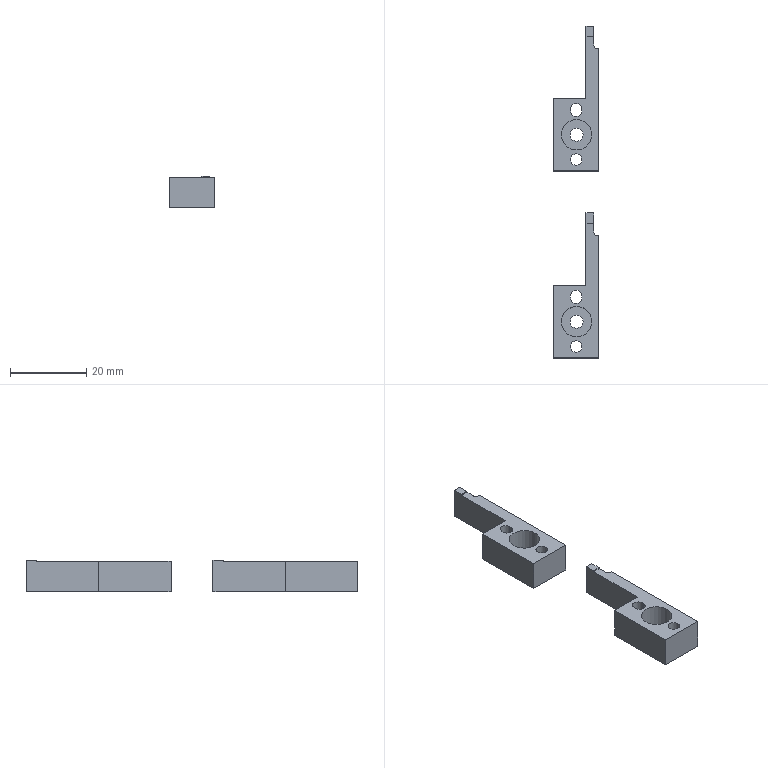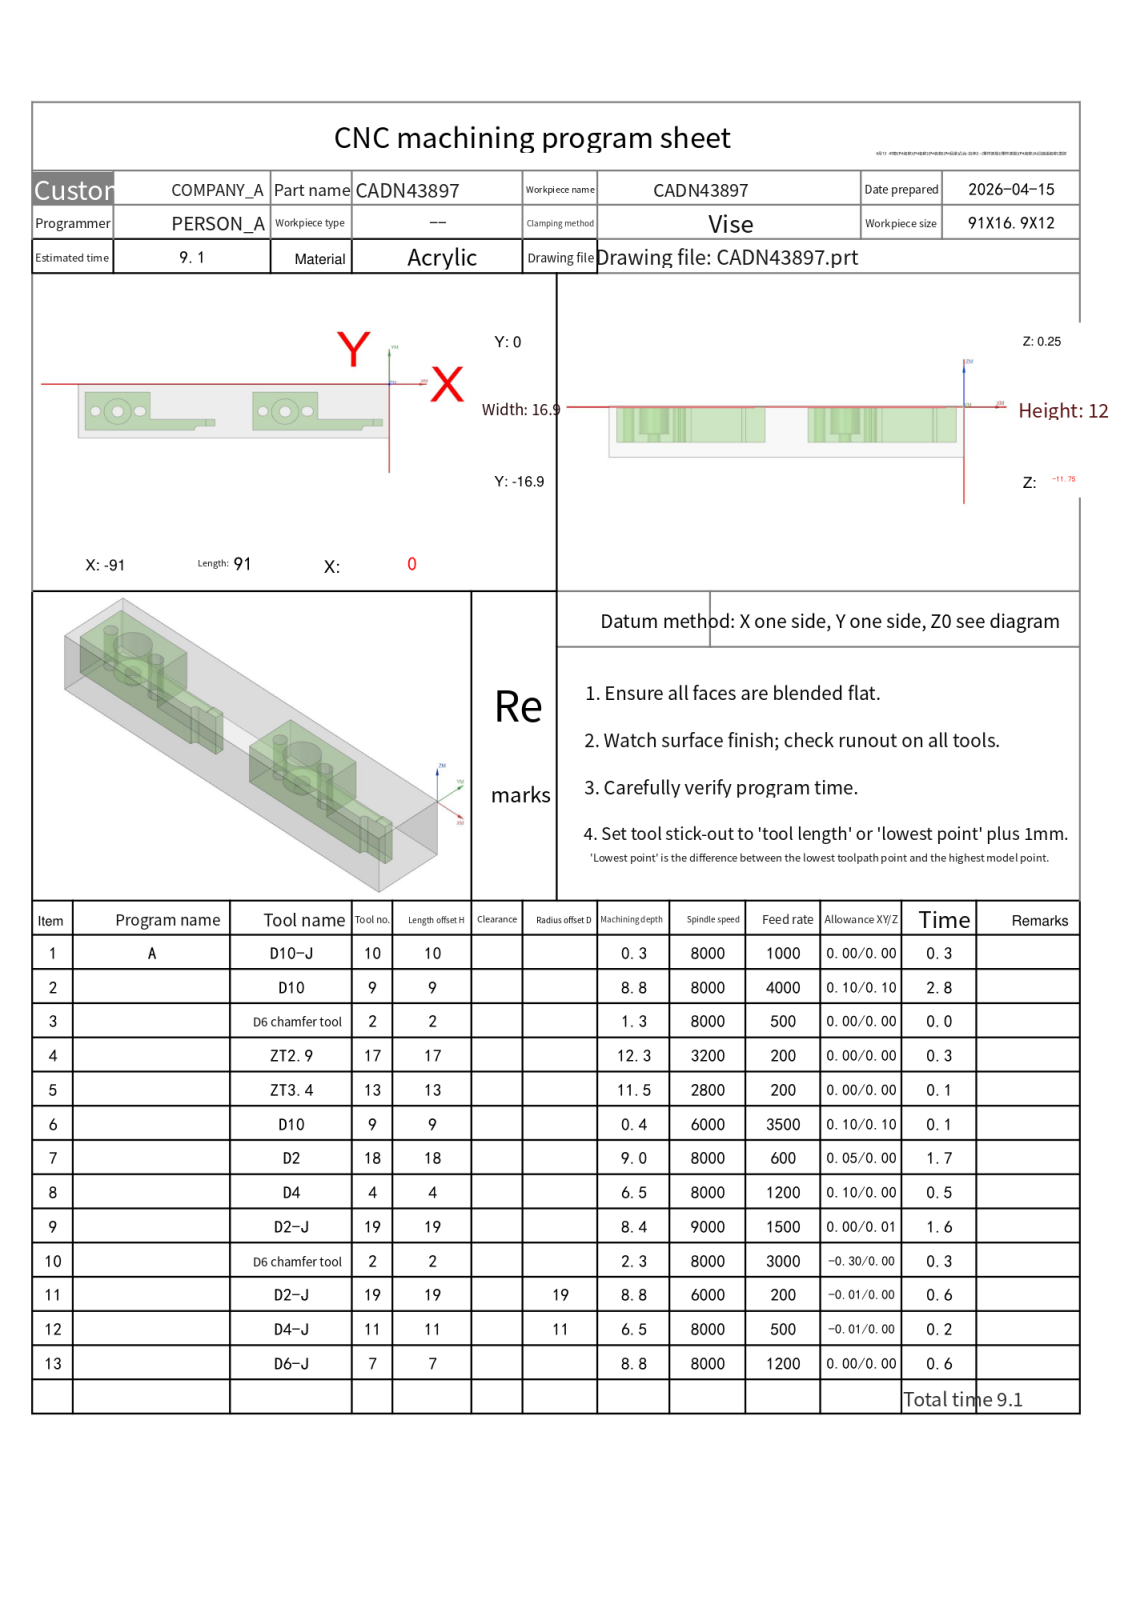NC program | NX | posted by the shop | part box 11.9 x 87 x 8.25 mm
Lines 3432 to 4498 of 9110:
N9 T19 M06
(D2-J  D=2. R=0. H=19 ce=0.00 di=0.01)
G00 G90 G54 X-68.246 Y-5.182 M03 S9000
G43 H19 Z20.
M08
Z.452
G01 X-68.256 Y-5.184 Z.338 F1200.
X-68.283 Y-5.191 Z.235
X-68.325 Y-5.203 Z.143
X-68.378 Y-5.221 Z.062
X-68.442 Y-5.245 Z-.009
X-68.512 Y-5.276 Z-.071
X-68.585 Y-5.314 Z-.125
X-68.661 Y-5.36 Z-.17
X-68.735 Y-5.414 Z-.207
X-68.805 Y-5.477 Z-.237
X-68.868 Y-5.549 Z-.26
X-68.922 Y-5.631 Z-.278
X-68.963 Y-5.723 Z-.289
X-68.99 Y-5.826 Z-.296
X-69. Y-5.941 Z-.298
Y-10.04 F1500.
X-64.901
X-64.887 Y-10.024 Z-.299
X-64.898 Y-9.979 Z-.3
X-64.932 Y-9.908 Z-.302
X-64.988 Y-9.813 Z-.305
X-65.207 Y-9.496 Z-.314
X-65.429 Y-9.2 Z-.324
X-65.728 Y-8.827 Z-.335
X-66.245 Y-8.237 Z-.355
X-66.712 Y-7.751 Z-.373
X-67.198 Y-7.284 Z-.39
X-67.787 Y-6.767 Z-.41
X-68.16 Y-6.469 Z-.422
X-68.456 Y-6.246 Z-.431
X-68.773 Y-6.028 Z-.441
X-68.868 Y-5.972 Z-.443
X-68.939 Y-5.938 Z-.446
X-68.984 Y-5.927 Z-.447
X-69. Y-5.941
Y-10.04
X-64.901
X-64.887 Y-10.024 Z-.448
X-64.898 Y-9.979 Z-.449
X-64.932 Y-9.908 Z-.451
X-64.988 Y-9.813 Z-.454
X-65.207 Y-9.496 Z-.463
X-65.429 Y-9.2 Z-.473
X-65.728 Y-8.827 Z-.485
X-66.245 Y-8.237 Z-.504
X-66.712 Y-7.751 Z-.522
X-67.198 Y-7.284 Z-.539
X-67.787 Y-6.767 Z-.559
X-68.16 Y-6.469 Z-.571
X-68.456 Y-6.246 Z-.58
X-68.773 Y-6.028 Z-.59
X-68.868 Y-5.972 Z-.593
X-68.939 Y-5.938 Z-.595
X-68.984 Y-5.927 Z-.596
X-69. Y-5.941
Y-10.04
X-64.901
X-64.887 Y-10.024 Z-.597
X-64.898 Y-9.979 Z-.598
X-64.932 Y-9.908 Z-.6
X-64.988 Y-9.813 Z-.603
X-65.207 Y-9.496 Z-.613
X-65.429 Y-9.2 Z-.622
X-65.728 Y-8.827 Z-.634
X-66.245 Y-8.237 Z-.654
X-66.712 Y-7.751 Z-.671
X-67.198 Y-7.284 Z-.688
X-67.787 Y-6.767 Z-.708
X-68.16 Y-6.469 Z-.72
X-68.456 Y-6.246 Z-.729
X-68.773 Y-6.028 Z-.739
X-68.868 Y-5.972 Z-.742
X-68.939 Y-5.938 Z-.744
X-68.984 Y-5.927 Z-.745
X-69. Y-5.941
Y-10.04
X-64.901
X-64.887 Y-10.024 Z-.746
X-64.898 Y-9.979 Z-.747
X-64.932 Y-9.908 Z-.749
X-64.988 Y-9.813 Z-.752
X-65.207 Y-9.496 Z-.762
X-65.429 Y-9.2 Z-.771
X-65.728 Y-8.827 Z-.783
X-66.245 Y-8.237 Z-.803
X-66.712 Y-7.751 Z-.82
X-67.198 Y-7.284 Z-.837
X-67.787 Y-6.767 Z-.857
X-68.16 Y-6.469 Z-.869
X-68.456 Y-6.246 Z-.878
X-68.773 Y-6.028 Z-.888
X-68.868 Y-5.972 Z-.891
X-68.939 Y-5.938 Z-.893
X-68.984 Y-5.927 Z-.894
X-69. Y-5.941 Z-.895
Y-10.04
X-64.901
X-64.887 Y-10.024
X-64.898 Y-9.979 Z-.896
X-64.932 Y-9.908 Z-.898
X-64.988 Y-9.813 Z-.901
X-65.207 Y-9.496 Z-.911
X-65.429 Y-9.2 Z-.92
X-65.728 Y-8.827 Z-.932
X-66.245 Y-8.237 Z-.952
X-66.712 Y-7.751 Z-.969
X-67.198 Y-7.284 Z-.986
X-67.787 Y-6.767 Z-1.006
X-68.16 Y-6.469 Z-1.018
X-68.456 Y-6.246 Z-1.027
X-68.773 Y-6.028 Z-1.037
X-68.868 Y-5.972 Z-1.04
X-68.939 Y-5.938 Z-1.042
X-68.984 Y-5.927 Z-1.043
X-69. Y-5.941 Z-1.044
Y-10.04
X-64.901
X-64.887 Y-10.024
X-64.898 Y-9.979 Z-1.045
X-64.932 Y-9.908 Z-1.047
X-64.988 Y-9.813 Z-1.05
X-65.207 Y-9.496 Z-1.06
X-65.429 Y-9.2 Z-1.069
X-65.728 Y-8.827 Z-1.081
X-66.245 Y-8.237 Z-1.101
X-66.712 Y-7.751 Z-1.118
X-67.198 Y-7.284 Z-1.136
X-67.787 Y-6.767 Z-1.155
X-68.16 Y-6.469 Z-1.167
X-68.456 Y-6.246 Z-1.177
X-68.773 Y-6.028 Z-1.186
X-68.868 Y-5.972 Z-1.189
X-68.939 Y-5.938 Z-1.191
X-68.984 Y-5.927 Z-1.192
X-69. Y-5.941 Z-1.193
Y-10.04
X-64.901
X-64.887 Y-10.024
X-64.898 Y-9.979 Z-1.194
X-64.932 Y-9.908 Z-1.197
X-64.988 Y-9.813 Z-1.199
X-65.207 Y-9.496 Z-1.209
X-65.429 Y-9.2 Z-1.218
X-65.728 Y-8.827 Z-1.23
X-66.245 Y-8.237 Z-1.25
X-66.712 Y-7.751 Z-1.267
X-67.198 Y-7.284 Z-1.285
X-67.787 Y-6.767 Z-1.305
X-68.16 Y-6.469 Z-1.316
X-68.456 Y-6.246 Z-1.326
X-68.773 Y-6.028 Z-1.335
X-68.868 Y-5.972 Z-1.338
X-68.939 Y-5.938 Z-1.34
X-68.984 Y-5.927 Z-1.341
X-69. Y-5.941 Z-1.342
Y-10.04
X-64.901
X-64.887 Y-10.024
X-64.898 Y-9.979 Z-1.344
X-64.932 Y-9.908 Z-1.346
X-64.988 Y-9.813 Z-1.348
X-65.207 Y-9.496 Z-1.358
X-65.429 Y-9.2 Z-1.367
X-65.728 Y-8.827 Z-1.379
X-66.245 Y-8.237 Z-1.399
X-66.712 Y-7.751 Z-1.416
X-67.198 Y-7.284 Z-1.434
X-67.787 Y-6.767 Z-1.454
X-68.16 Y-6.469 Z-1.466
X-68.456 Y-6.246 Z-1.475
X-68.773 Y-6.028 Z-1.484
X-68.868 Y-5.972 Z-1.487
X-68.939 Y-5.938 Z-1.489
X-68.984 Y-5.927 Z-1.49
X-69. Y-5.941 Z-1.491
Y-10.04
X-64.901
X-64.887 Y-10.024
X-64.898 Y-9.979 Z-1.493
X-64.932 Y-9.908 Z-1.495
X-64.988 Y-9.813 Z-1.498
X-65.207 Y-9.496 Z-1.507
X-65.429 Y-9.2 Z-1.516
X-65.728 Y-8.827 Z-1.528
X-66.245 Y-8.237 Z-1.548
X-66.712 Y-7.751 Z-1.565
X-67.198 Y-7.284 Z-1.583
X-67.787 Y-6.767 Z-1.603
X-68.16 Y-6.469 Z-1.615
X-68.456 Y-6.246 Z-1.624
X-68.773 Y-6.028 Z-1.633
X-68.868 Y-5.972 Z-1.636
X-68.939 Y-5.938 Z-1.638
X-68.984 Y-5.927 Z-1.64
X-69. Y-5.941
Y-10.04
X-64.901
X-64.887 Y-10.024
X-64.898 Y-9.979 Z-1.642
X-64.932 Y-9.908 Z-1.644
X-64.988 Y-9.813 Z-1.647
X-65.207 Y-9.496 Z-1.656
X-65.429 Y-9.2 Z-1.665
X-65.728 Y-8.827 Z-1.677
X-66.245 Y-8.237 Z-1.697
X-66.712 Y-7.751 Z-1.715
X-67.198 Y-7.284 Z-1.732
X-67.787 Y-6.767 Z-1.752
X-68.16 Y-6.469 Z-1.764
X-68.456 Y-6.246 Z-1.773
X-68.773 Y-6.028 Z-1.782
X-68.868 Y-5.972 Z-1.785
X-68.939 Y-5.938 Z-1.787
X-68.984 Y-5.927 Z-1.789
X-69. Y-5.941
Y-10.04
X-64.901
X-64.887 Y-10.024 Z-1.79
X-64.898 Y-9.979 Z-1.791
X-64.932 Y-9.908 Z-1.793
X-64.988 Y-9.813 Z-1.796
X-65.207 Y-9.496 Z-1.805
X-65.429 Y-9.2 Z-1.814
X-65.728 Y-8.827 Z-1.826
X-66.245 Y-8.237 Z-1.846
X-66.712 Y-7.751 Z-1.864
X-67.198 Y-7.284 Z-1.881
X-67.787 Y-6.767 Z-1.901
X-68.16 Y-6.469 Z-1.913
X-68.456 Y-6.246 Z-1.922
X-68.773 Y-6.028 Z-1.932
X-68.868 Y-5.972 Z-1.934
X-68.939 Y-5.938 Z-1.936
X-68.984 Y-5.927 Z-1.938
X-69. Y-5.941
Y-10.04
X-64.901
X-64.887 Y-10.024 Z-1.939
X-64.898 Y-9.979 Z-1.94
X-64.932 Y-9.908 Z-1.942
X-64.988 Y-9.813 Z-1.945
X-65.207 Y-9.496 Z-1.954
X-65.429 Y-9.2 Z-1.964
X-65.728 Y-8.827 Z-1.975
X-66.245 Y-8.237 Z-1.995
X-66.712 Y-7.751 Z-2.013
X-67.198 Y-7.284 Z-2.03
X-67.787 Y-6.767 Z-2.05
X-68.16 Y-6.469 Z-2.062
X-68.456 Y-6.246 Z-2.071
X-68.773 Y-6.028 Z-2.081
X-68.868 Y-5.972 Z-2.083
X-68.939 Y-5.938 Z-2.086
X-68.984 Y-5.927 Z-2.087
X-69. Y-5.941
Y-10.04
X-64.901
X-64.887 Y-10.024 Z-2.088
X-64.898 Y-9.979 Z-2.089
X-64.932 Y-9.908 Z-2.091
X-64.988 Y-9.813 Z-2.094
X-65.207 Y-9.496 Z-2.103
X-65.429 Y-9.2 Z-2.113
X-65.728 Y-8.827 Z-2.125
X-66.245 Y-8.237 Z-2.144
X-66.712 Y-7.751 Z-2.162
X-67.198 Y-7.284 Z-2.179
X-67.787 Y-6.767 Z-2.199
X-68.16 Y-6.469 Z-2.211
X-68.456 Y-6.246 Z-2.22
X-68.773 Y-6.028 Z-2.23
X-68.868 Y-5.972 Z-2.233
X-68.939 Y-5.938 Z-2.235
X-68.984 Y-5.927 Z-2.236
X-69. Y-5.941
Y-10.04
X-64.901
X-64.887 Y-10.024 Z-2.237
X-64.898 Y-9.979 Z-2.238
X-64.932 Y-9.908 Z-2.24
X-64.988 Y-9.813 Z-2.243
X-65.207 Y-9.496 Z-2.253
X-65.429 Y-9.2 Z-2.262
X-65.728 Y-8.827 Z-2.274
X-66.245 Y-8.237 Z-2.294
X-66.712 Y-7.751 Z-2.311
X-67.198 Y-7.284 Z-2.328
X-67.787 Y-6.767 Z-2.348
X-68.16 Y-6.469 Z-2.36
X-68.456 Y-6.246 Z-2.369
X-68.773 Y-6.028 Z-2.379
X-68.868 Y-5.972 Z-2.382
X-68.939 Y-5.938 Z-2.384
X-68.984 Y-5.927 Z-2.385
X-69. Y-5.941
Y-10.04
X-64.901
X-64.887 Y-10.024 Z-2.386
X-64.898 Y-9.979 Z-2.387
X-64.932 Y-9.908 Z-2.389
X-64.988 Y-9.813 Z-2.392
X-65.207 Y-9.496 Z-2.402
X-65.429 Y-9.2 Z-2.411
X-65.728 Y-8.827 Z-2.423
X-66.245 Y-8.237 Z-2.443
X-66.712 Y-7.751 Z-2.46
X-67.198 Y-7.284 Z-2.477
X-67.787 Y-6.767 Z-2.497
X-68.16 Y-6.469 Z-2.509
X-68.456 Y-6.246 Z-2.518
X-68.773 Y-6.028 Z-2.528
X-68.868 Y-5.972 Z-2.531
X-68.939 Y-5.938 Z-2.533
X-68.984 Y-5.927 Z-2.534
X-69. Y-5.941 Z-2.535
Y-10.04
X-64.901
X-64.887 Y-10.024
X-64.898 Y-9.979 Z-2.536
X-64.932 Y-9.908 Z-2.538
X-64.988 Y-9.813 Z-2.541
X-65.207 Y-9.496 Z-2.551
X-65.429 Y-9.2 Z-2.56
X-65.728 Y-8.827 Z-2.572
X-66.245 Y-8.237 Z-2.592
X-66.712 Y-7.751 Z-2.609
X-67.198 Y-7.284 Z-2.626
X-67.787 Y-6.767 Z-2.646
X-68.16 Y-6.469 Z-2.658
X-68.456 Y-6.246 Z-2.667
X-68.773 Y-6.028 Z-2.677
X-68.868 Y-5.972 Z-2.68
X-68.939 Y-5.938 Z-2.682
X-68.984 Y-5.927 Z-2.683
X-69. Y-5.941 Z-2.684
Y-10.04
X-64.901
X-64.887 Y-10.024
X-64.898 Y-9.979 Z-2.685
X-64.932 Y-9.908 Z-2.687
X-64.988 Y-9.813 Z-2.69
X-65.207 Y-9.496 Z-2.7
X-65.429 Y-9.2 Z-2.709
X-65.728 Y-8.827 Z-2.721
X-66.245 Y-8.237 Z-2.741
X-66.712 Y-7.751 Z-2.758
X-67.198 Y-7.284 Z-2.776
X-67.787 Y-6.767 Z-2.795
X-68.16 Y-6.469 Z-2.807
X-68.456 Y-6.246 Z-2.817
X-68.773 Y-6.028 Z-2.826
X-68.868 Y-5.972 Z-2.829
X-68.939 Y-5.938 Z-2.831
X-68.984 Y-5.927 Z-2.832
X-69. Y-5.941 Z-2.833
Y-10.04
X-64.901
X-64.887 Y-10.024
X-64.898 Y-9.979 Z-2.834
X-64.932 Y-9.908 Z-2.837
X-64.988 Y-9.813 Z-2.839
X-65.207 Y-9.496 Z-2.849
X-65.429 Y-9.2 Z-2.858
X-65.728 Y-8.827 Z-2.87
X-66.245 Y-8.237 Z-2.89
X-66.712 Y-7.751 Z-2.907
X-67.198 Y-7.284 Z-2.925
X-67.787 Y-6.767 Z-2.945
X-68.16 Y-6.469 Z-2.956
X-68.456 Y-6.246 Z-2.966
X-68.773 Y-6.028 Z-2.975
X-68.868 Y-5.972 Z-2.978
X-68.939 Y-5.938 Z-2.98
X-68.984 Y-5.927 Z-2.981
X-69. Y-5.941 Z-2.982
Y-10.04
X-64.901
X-64.887 Y-10.024
X-64.898 Y-9.979 Z-2.984
X-64.932 Y-9.908 Z-2.986
X-64.988 Y-9.813 Z-2.988
X-65.207 Y-9.496 Z-2.998
X-65.429 Y-9.2 Z-3.007
X-65.728 Y-8.827 Z-3.019
X-66.245 Y-8.237 Z-3.039
X-66.712 Y-7.751 Z-3.056
X-67.198 Y-7.284 Z-3.074
X-67.787 Y-6.767 Z-3.094
X-68.16 Y-6.469 Z-3.106
X-68.456 Y-6.246 Z-3.115
X-68.773 Y-6.028 Z-3.124
X-68.868 Y-5.972 Z-3.127
X-68.939 Y-5.938 Z-3.129
X-68.984 Y-5.927 Z-3.13
X-69. Y-5.941 Z-3.131
Y-10.04
X-64.901
X-64.887 Y-10.024
X-64.898 Y-9.979 Z-3.133
X-64.932 Y-9.908 Z-3.135
X-64.988 Y-9.813 Z-3.138
X-65.207 Y-9.496 Z-3.147
X-65.429 Y-9.2 Z-3.156
X-65.728 Y-8.827 Z-3.168
X-66.245 Y-8.237 Z-3.188
X-66.712 Y-7.751 Z-3.205
X-67.198 Y-7.284 Z-3.223
X-67.787 Y-6.767 Z-3.243
X-68.16 Y-6.469 Z-3.255
X-68.456 Y-6.246 Z-3.264
X-68.773 Y-6.028 Z-3.273
X-68.868 Y-5.972 Z-3.276
X-68.939 Y-5.938 Z-3.278
X-68.984 Y-5.927 Z-3.28
X-69. Y-5.941
Y-10.04
X-64.901
X-64.887 Y-10.024
X-64.898 Y-9.979 Z-3.282
X-64.932 Y-9.908 Z-3.284
X-64.988 Y-9.813 Z-3.287
X-65.207 Y-9.496 Z-3.296
X-65.429 Y-9.2 Z-3.305
X-65.728 Y-8.827 Z-3.317
X-66.245 Y-8.237 Z-3.337
X-66.712 Y-7.751 Z-3.355
X-67.198 Y-7.284 Z-3.372
X-67.787 Y-6.767 Z-3.392
X-68.16 Y-6.469 Z-3.404
X-68.456 Y-6.246 Z-3.413
X-68.773 Y-6.028 Z-3.422
X-68.868 Y-5.972 Z-3.425
X-68.939 Y-5.938 Z-3.427
X-68.984 Y-5.927 Z-3.429
X-69. Y-5.941
Y-10.04
X-64.901
X-64.887 Y-10.024 Z-3.43
X-64.898 Y-9.979 Z-3.431
X-64.932 Y-9.908 Z-3.433
X-64.988 Y-9.813 Z-3.436
X-65.207 Y-9.496 Z-3.445
X-65.429 Y-9.2 Z-3.454
X-65.728 Y-8.827 Z-3.466
X-66.245 Y-8.237 Z-3.486
X-66.712 Y-7.751 Z-3.504
X-67.198 Y-7.284 Z-3.521
X-67.787 Y-6.767 Z-3.541
X-68.16 Y-6.469 Z-3.553
X-68.456 Y-6.246 Z-3.562
X-68.773 Y-6.028 Z-3.572
X-68.868 Y-5.972 Z-3.574
X-68.939 Y-5.938 Z-3.576
X-68.984 Y-5.927 Z-3.578
X-69. Y-5.941
Y-10.04
X-64.901
X-64.887 Y-10.024 Z-3.579
X-64.898 Y-9.979 Z-3.58
X-64.932 Y-9.908 Z-3.582
X-64.988 Y-9.813 Z-3.585
X-65.207 Y-9.496 Z-3.594
X-65.429 Y-9.2 Z-3.604
X-65.728 Y-8.827 Z-3.615
X-66.245 Y-8.237 Z-3.635
X-66.712 Y-7.751 Z-3.653
X-67.198 Y-7.284 Z-3.67
X-67.787 Y-6.767 Z-3.69
X-68.16 Y-6.469 Z-3.702
X-68.456 Y-6.246 Z-3.711
X-68.773 Y-6.028 Z-3.721
X-68.868 Y-5.972 Z-3.723
X-68.939 Y-5.938 Z-3.726
X-68.984 Y-5.927 Z-3.727
X-69. Y-5.941
Y-10.04
X-64.901
X-64.887 Y-10.024 Z-3.728
X-64.898 Y-9.979 Z-3.729
X-64.932 Y-9.908 Z-3.731
X-64.988 Y-9.813 Z-3.734
X-65.207 Y-9.496 Z-3.743
X-65.429 Y-9.2 Z-3.753
X-65.728 Y-8.827 Z-3.765
X-66.245 Y-8.237 Z-3.784
X-66.712 Y-7.751 Z-3.802
X-67.198 Y-7.284 Z-3.819
X-67.787 Y-6.767 Z-3.839
X-68.16 Y-6.469 Z-3.851
X-68.456 Y-6.246 Z-3.86
X-68.773 Y-6.028 Z-3.87
X-68.868 Y-5.972 Z-3.873
X-68.939 Y-5.938 Z-3.875
X-68.984 Y-5.927 Z-3.876
X-69. Y-5.941
Y-10.04
X-64.901
X-64.887 Y-10.024 Z-3.877
X-64.898 Y-9.979 Z-3.878
X-64.932 Y-9.908 Z-3.88
X-64.988 Y-9.813 Z-3.883
X-65.207 Y-9.496 Z-3.893
X-65.429 Y-9.2 Z-3.902
X-65.728 Y-8.827 Z-3.914
X-66.245 Y-8.237 Z-3.934
X-66.712 Y-7.751 Z-3.951
X-67.198 Y-7.284 Z-3.968
X-67.787 Y-6.767 Z-3.988
X-68.16 Y-6.469 Z-4.
X-68.456 Y-6.246 Z-4.009
X-68.773 Y-6.028 Z-4.019
X-68.868 Y-5.972 Z-4.022
X-68.939 Y-5.938 Z-4.024
X-68.984 Y-5.927 Z-4.025
X-69. Y-5.941
Y-10.04
X-64.901
X-64.887 Y-10.024 Z-4.026
X-64.898 Y-9.979 Z-4.027
X-64.932 Y-9.908 Z-4.029
X-64.988 Y-9.813 Z-4.032
X-65.207 Y-9.496 Z-4.042
X-65.429 Y-9.2 Z-4.051
X-65.728 Y-8.827 Z-4.063
X-66.245 Y-8.237 Z-4.083
X-66.712 Y-7.751 Z-4.1
X-67.198 Y-7.284 Z-4.117
X-67.787 Y-6.767 Z-4.137
X-68.16 Y-6.469 Z-4.149
X-68.456 Y-6.246 Z-4.158
X-68.773 Y-6.028 Z-4.168
X-68.868 Y-5.972 Z-4.171
X-68.939 Y-5.938 Z-4.173
X-68.984 Y-5.927 Z-4.174
X-69. Y-5.941 Z-4.175
Y-10.04
X-64.901
X-64.887 Y-10.024
X-64.898 Y-9.979 Z-4.176
X-64.932 Y-9.908 Z-4.178
X-64.988 Y-9.813 Z-4.181
X-65.207 Y-9.496 Z-4.191
X-65.429 Y-9.2 Z-4.2
X-65.728 Y-8.827 Z-4.212
X-66.245 Y-8.237 Z-4.232
X-66.712 Y-7.751 Z-4.249
X-67.198 Y-7.284 Z-4.266
X-67.787 Y-6.767 Z-4.286
X-68.16 Y-6.469 Z-4.298
X-68.456 Y-6.246 Z-4.307
X-68.773 Y-6.028 Z-4.317
X-68.868 Y-5.972 Z-4.32
X-68.939 Y-5.938 Z-4.322
X-68.984 Y-5.927 Z-4.323
X-69. Y-5.941 Z-4.324
Y-10.04
X-64.901
X-64.887 Y-10.024
X-64.898 Y-9.979 Z-4.325
X-64.932 Y-9.908 Z-4.327
X-64.988 Y-9.813 Z-4.33
X-65.207 Y-9.496 Z-4.34
X-65.429 Y-9.2 Z-4.349
X-65.728 Y-8.827 Z-4.361
X-66.245 Y-8.237 Z-4.381
X-66.712 Y-7.751 Z-4.398
X-67.198 Y-7.284 Z-4.416
X-67.787 Y-6.767 Z-4.435
X-68.16 Y-6.469 Z-4.447
X-68.456 Y-6.246 Z-4.457
X-68.773 Y-6.028 Z-4.466
X-68.868 Y-5.972 Z-4.469
X-68.939 Y-5.938 Z-4.471
X-68.984 Y-5.927 Z-4.472
X-69. Y-5.941 Z-4.473
Y-10.04
X-64.901
X-64.887 Y-10.024
X-64.898 Y-9.979 Z-4.474
X-64.932 Y-9.908 Z-4.477
X-64.988 Y-9.813 Z-4.479
X-65.207 Y-9.496 Z-4.489
X-65.429 Y-9.2 Z-4.498
X-65.728 Y-8.827 Z-4.51
X-66.245 Y-8.237 Z-4.53
X-66.712 Y-7.751 Z-4.547
X-67.198 Y-7.284 Z-4.565
X-67.787 Y-6.767 Z-4.585
X-68.16 Y-6.469 Z-4.596
X-68.456 Y-6.246 Z-4.606
X-68.773 Y-6.028 Z-4.615
X-68.868 Y-5.972 Z-4.618
X-68.939 Y-5.938 Z-4.62
X-68.984 Y-5.927 Z-4.621
X-69. Y-5.941 Z-4.622
Y-10.04
X-64.901
X-64.887 Y-10.024
X-64.898 Y-9.979 Z-4.624
X-64.932 Y-9.908 Z-4.626
X-64.988 Y-9.813 Z-4.628
X-65.207 Y-9.496 Z-4.638
X-65.429 Y-9.2 Z-4.647
X-65.728 Y-8.827 Z-4.659
X-66.245 Y-8.237 Z-4.679
X-66.712 Y-7.751 Z-4.696
X-67.198 Y-7.284 Z-4.714
X-67.787 Y-6.767 Z-4.734
X-68.16 Y-6.469 Z-4.746
X-68.456 Y-6.246 Z-4.755
X-68.773 Y-6.028 Z-4.764
X-68.868 Y-5.972 Z-4.767
X-68.939 Y-5.938 Z-4.769
X-68.984 Y-5.927 Z-4.77
X-69. Y-5.941 Z-4.771
Y-10.04
X-64.901
X-64.887 Y-10.024
X-64.898 Y-9.979 Z-4.773
X-64.932 Y-9.908 Z-4.775
X-64.988 Y-9.813 Z-4.778
X-65.207 Y-9.496 Z-4.787
X-65.429 Y-9.2 Z-4.796
X-65.728 Y-8.827 Z-4.808
X-66.245 Y-8.237 Z-4.828
X-66.712 Y-7.751 Z-4.845
X-67.198 Y-7.284 Z-4.863
X-67.787 Y-6.767 Z-4.883
X-68.16 Y-6.469 Z-4.895
X-68.456 Y-6.246 Z-4.904
X-68.773 Y-6.028 Z-4.913
X-68.868 Y-5.972 Z-4.916
X-68.939 Y-5.938 Z-4.918
X-68.984 Y-5.927 Z-4.92
X-69. Y-5.941
Y-10.04
X-64.901
X-64.887 Y-10.024
X-64.898 Y-9.979 Z-4.922
X-64.932 Y-9.908 Z-4.924
X-64.988 Y-9.813 Z-4.927
X-65.207 Y-9.496 Z-4.936
X-65.429 Y-9.2 Z-4.945
X-65.728 Y-8.827 Z-4.957
X-66.245 Y-8.237 Z-4.977
X-66.712 Y-7.751 Z-4.995
X-67.198 Y-7.284 Z-5.012
X-67.787 Y-6.767 Z-5.032
X-68.16 Y-6.469 Z-5.044
X-68.456 Y-6.246 Z-5.053
X-68.773 Y-6.028 Z-5.062
X-68.868 Y-5.972 Z-5.065
X-68.939 Y-5.938 Z-5.067
X-68.984 Y-5.927 Z-5.069
X-69. Y-5.941
Y-10.04
X-64.901
X-64.887 Y-10.024 Z-5.07
X-64.898 Y-9.979 Z-5.071
X-64.932 Y-9.908 Z-5.073
X-64.988 Y-9.813 Z-5.076
X-65.207 Y-9.496 Z-5.085
X-65.429 Y-9.2 Z-5.094
X-65.728 Y-8.827 Z-5.106
X-66.245 Y-8.237 Z-5.126
X-66.712 Y-7.751 Z-5.144
X-67.198 Y-7.284 Z-5.161
X-67.787 Y-6.767 Z-5.181
X-68.16 Y-6.469 Z-5.193
X-68.456 Y-6.246 Z-5.202
X-68.773 Y-6.028 Z-5.212
X-68.868 Y-5.972 Z-5.214
X-68.939 Y-5.938 Z-5.216
X-68.984 Y-5.927 Z-5.218
X-69. Y-5.941
Y-10.04
X-64.901
X-64.887 Y-10.024 Z-5.219
X-64.898 Y-9.979 Z-5.22
X-64.932 Y-9.908 Z-5.222
X-64.988 Y-9.813 Z-5.225
X-65.207 Y-9.496 Z-5.234
X-65.429 Y-9.2 Z-5.244
X-65.728 Y-8.827 Z-5.255
X-66.245 Y-8.237 Z-5.275
X-66.712 Y-7.751 Z-5.293
X-67.198 Y-7.284 Z-5.31
X-67.787 Y-6.767 Z-5.33
X-68.16 Y-6.469 Z-5.342
X-68.456 Y-6.246 Z-5.351
X-68.773 Y-6.028 Z-5.361
X-68.868 Y-5.972 Z-5.363
X-68.939 Y-5.938 Z-5.366
X-68.984 Y-5.927 Z-5.367
X-69. Y-5.941
Y-10.04
X-64.901
X-64.887 Y-10.024 Z-5.368
X-64.898 Y-9.979 Z-5.369
X-64.932 Y-9.908 Z-5.371
X-64.988 Y-9.813 Z-5.374
X-65.207 Y-9.496 Z-5.383
X-65.429 Y-9.2 Z-5.393
X-65.728 Y-8.827 Z-5.405
X-66.245 Y-8.237 Z-5.424
X-66.712 Y-7.751 Z-5.442
X-67.198 Y-7.284 Z-5.459
X-67.787 Y-6.767 Z-5.479
X-68.16 Y-6.469 Z-5.491
X-68.456 Y-6.246 Z-5.5
X-68.773 Y-6.028 Z-5.51
X-68.868 Y-5.972 Z-5.513
X-68.939 Y-5.938 Z-5.515
X-68.984 Y-5.927 Z-5.516
X-69. Y-5.941
Y-10.04
X-64.901
X-64.887 Y-10.024 Z-5.517
X-64.898 Y-9.979 Z-5.518
X-64.932 Y-9.908 Z-5.52
X-64.988 Y-9.813 Z-5.523
X-65.207 Y-9.496 Z-5.533
X-65.429 Y-9.2 Z-5.542
X-65.728 Y-8.827 Z-5.554
X-66.245 Y-8.237 Z-5.574
X-66.712 Y-7.751 Z-5.591
X-67.198 Y-7.284 Z-5.608
X-67.787 Y-6.767 Z-5.628
X-68.16 Y-6.469 Z-5.64
X-68.456 Y-6.246 Z-5.649
X-68.773 Y-6.028 Z-5.659
X-68.868 Y-5.972 Z-5.662
X-68.939 Y-5.938 Z-5.664
X-68.984 Y-5.927 Z-5.665
X-69. Y-5.941
Y-10.04
X-64.901
X-64.887 Y-10.024 Z-5.666
X-64.898 Y-9.979 Z-5.667
X-64.932 Y-9.908 Z-5.669
X-64.988 Y-9.813 Z-5.672
X-65.207 Y-9.496 Z-5.682
X-65.429 Y-9.2 Z-5.691
X-65.728 Y-8.827 Z-5.703
X-66.245 Y-8.237 Z-5.723
X-66.712 Y-7.751 Z-5.74
X-67.198 Y-7.284 Z-5.757
X-67.787 Y-6.767 Z-5.777
X-68.16 Y-6.469 Z-5.789
X-68.456 Y-6.246 Z-5.798
X-68.773 Y-6.028 Z-5.808
X-68.868 Y-5.972 Z-5.811
X-68.939 Y-5.938 Z-5.813
X-68.984 Y-5.927 Z-5.814
X-69. Y-5.941 Z-5.815
Y-10.04
X-64.901
X-64.887 Y-10.024
X-64.898 Y-9.979 Z-5.816
X-64.932 Y-9.908 Z-5.818
X-64.988 Y-9.813 Z-5.821
X-65.207 Y-9.496 Z-5.831
X-65.429 Y-9.2 Z-5.84
X-65.728 Y-8.827 Z-5.852
X-66.245 Y-8.237 Z-5.872
X-66.712 Y-7.751 Z-5.889
X-67.198 Y-7.284 Z-5.906
X-67.787 Y-6.767 Z-5.926
X-68.16 Y-6.469 Z-5.938
X-68.456 Y-6.246 Z-5.947
X-68.773 Y-6.028 Z-5.957
X-68.868 Y-5.972 Z-5.96
X-68.939 Y-5.938 Z-5.962
X-68.984 Y-5.927 Z-5.963
X-69. Y-5.941 Z-5.964
Y-10.04
X-64.901
X-64.887 Y-10.024
X-64.898 Y-9.979 Z-5.965
X-64.932 Y-9.908 Z-5.967
X-64.988 Y-9.813 Z-5.97
X-65.207 Y-9.496 Z-5.98
X-65.429 Y-9.2 Z-5.989
X-65.728 Y-8.827 Z-6.001
X-66.245 Y-8.237 Z-6.021
X-66.712 Y-7.751 Z-6.038
X-67.198 Y-7.284 Z-6.056
X-67.787 Y-6.767 Z-6.075
X-68.16 Y-6.469 Z-6.087
X-68.456 Y-6.246 Z-6.097
X-68.773 Y-6.028 Z-6.106
X-68.868 Y-5.972 Z-6.109
X-68.939 Y-5.938 Z-6.111
X-68.984 Y-5.927 Z-6.112
X-69. Y-5.941 Z-6.113
Y-10.04
X-64.901
X-64.887 Y-10.024
X-64.898 Y-9.979 Z-6.114
X-64.932 Y-9.908 Z-6.117
X-64.988 Y-9.813 Z-6.119
X-65.207 Y-9.496 Z-6.129
X-65.429 Y-9.2 Z-6.138
X-65.728 Y-8.827 Z-6.15
X-66.245 Y-8.237 Z-6.17
X-66.712 Y-7.751 Z-6.187
X-67.198 Y-7.284 Z-6.205
X-67.787 Y-6.767 Z-6.225
X-68.16 Y-6.469 Z-6.236
X-68.456 Y-6.246 Z-6.246
X-68.773 Y-6.028 Z-6.255
X-68.868 Y-5.972 Z-6.258
X-68.939 Y-5.938 Z-6.26
X-68.984 Y-5.927 Z-6.261
X-69. Y-5.941 Z-6.262
Y-10.04
X-64.901
X-64.887 Y-10.024
X-64.898 Y-9.979 Z-6.264
X-64.932 Y-9.908 Z-6.266
X-64.988 Y-9.813 Z-6.268
X-65.207 Y-9.496 Z-6.278
X-65.429 Y-9.2 Z-6.287
X-65.728 Y-8.827 Z-6.299
X-66.245 Y-8.237 Z-6.319
X-66.712 Y-7.751 Z-6.336
X-67.198 Y-7.284 Z-6.354
X-67.787 Y-6.767 Z-6.374
X-68.16 Y-6.469 Z-6.386
X-68.456 Y-6.246 Z-6.395
X-68.773 Y-6.028 Z-6.404
X-68.868 Y-5.972 Z-6.407
X-68.939 Y-5.938 Z-6.409
X-68.984 Y-5.927 Z-6.41
X-69. Y-5.941 Z-6.411
Y-10.04
X-64.901
X-64.887 Y-10.024
X-64.898 Y-9.979 Z-6.413
X-64.932 Y-9.908 Z-6.415
X-64.988 Y-9.813 Z-6.418
X-65.207 Y-9.496 Z-6.427
X-65.429 Y-9.2 Z-6.436
X-65.728 Y-8.827 Z-6.448
X-66.245 Y-8.237 Z-6.468
X-66.712 Y-7.751 Z-6.485
X-67.198 Y-7.284 Z-6.503
X-67.787 Y-6.767 Z-6.523
X-68.16 Y-6.469 Z-6.535
X-68.456 Y-6.246 Z-6.544
X-68.773 Y-6.028 Z-6.553
X-68.868 Y-5.972 Z-6.556
X-68.939 Y-5.938 Z-6.558
X-68.984 Y-5.927 Z-6.56
X-69. Y-5.941
Y-10.04
X-64.901
X-64.887 Y-10.024
X-64.898 Y-9.979 Z-6.562
X-64.932 Y-9.908 Z-6.564
X-64.988 Y-9.813 Z-6.567
X-65.207 Y-9.496 Z-6.576
X-65.429 Y-9.2 Z-6.585
X-65.728 Y-8.827 Z-6.597
X-66.245 Y-8.237 Z-6.617
X-66.712 Y-7.751 Z-6.635
X-67.198 Y-7.284 Z-6.652
X-67.787 Y-6.767 Z-6.672
X-68.16 Y-6.469 Z-6.684
X-68.456 Y-6.246 Z-6.693
X-68.773 Y-6.028 Z-6.702
X-68.868 Y-5.972 Z-6.705
X-68.939 Y-5.938 Z-6.707
X-68.984 Y-5.927 Z-6.709
X-69. Y-5.941
Y-10.04
X-64.901
X-64.887 Y-10.024 Z-6.71
X-64.898 Y-9.979 Z-6.711
X-64.932 Y-9.908 Z-6.713
X-64.988 Y-9.813 Z-6.716
X-65.207 Y-9.496 Z-6.725
X-65.429 Y-9.2 Z-6.734
X-65.728 Y-8.827 Z-6.746
X-66.245 Y-8.237 Z-6.766
X-66.712 Y-7.751 Z-6.784
X-67.198 Y-7.284 Z-6.801
X-67.787 Y-6.767 Z-6.821
X-68.16 Y-6.469 Z-6.833
X-68.456 Y-6.246 Z-6.842
X-68.773 Y-6.028 Z-6.852
X-68.868 Y-5.972 Z-6.854
X-68.939 Y-5.938 Z-6.856
X-68.984 Y-5.927 Z-6.858
X-69. Y-5.941
Y-10.04
X-64.901
X-64.887 Y-10.024 Z-6.859
X-64.898 Y-9.979 Z-6.86
X-64.932 Y-9.908 Z-6.862
X-64.988 Y-9.813 Z-6.865
X-65.207 Y-9.496 Z-6.874
X-65.429 Y-9.2 Z-6.884
X-65.728 Y-8.827 Z-6.895
X-66.245 Y-8.237 Z-6.915
X-66.712 Y-7.751 Z-6.933
X-67.198 Y-7.284 Z-6.95
X-67.787 Y-6.767 Z-6.97
X-68.16 Y-6.469 Z-6.982
X-68.456 Y-6.246 Z-6.991
X-68.773 Y-6.028 Z-7.001
X-68.868 Y-5.972 Z-7.003
X-68.939 Y-5.938 Z-7.006
X-68.984 Y-5.927 Z-7.007
X-69. Y-5.941
Y-10.04
X-64.901
X-64.887 Y-10.024 Z-7.008
X-64.898 Y-9.979 Z-7.009
X-64.932 Y-9.908 Z-7.011
X-64.988 Y-9.813 Z-7.014
X-65.207 Y-9.496 Z-7.023
X-65.429 Y-9.2 Z-7.033
X-65.728 Y-8.827 Z-7.045
X-66.245 Y-8.237 Z-7.064
X-66.712 Y-7.751 Z-7.082
X-67.198 Y-7.284 Z-7.099
X-67.787 Y-6.767 Z-7.119
X-68.16 Y-6.469 Z-7.131
X-68.456 Y-6.246 Z-7.14
X-68.773 Y-6.028 Z-7.15
X-68.868 Y-5.972 Z-7.153
X-68.939 Y-5.938 Z-7.155
X-68.984 Y-5.927 Z-7.156
X-69. Y-5.941
Y-10.04
X-64.901
X-64.887 Y-10.024 Z-7.157
X-64.898 Y-9.979 Z-7.158
X-64.932 Y-9.908 Z-7.16
X-64.988 Y-9.813 Z-7.163
X-65.207 Y-9.496 Z-7.173
X-65.429 Y-9.2 Z-7.182
X-65.728 Y-8.827 Z-7.194
X-66.245 Y-8.237 Z-7.214
X-66.712 Y-7.751 Z-7.231
X-67.198 Y-7.284 Z-7.248
X-67.787 Y-6.767 Z-7.268
X-68.16 Y-6.469 Z-7.28
X-68.456 Y-6.246 Z-7.289
X-68.773 Y-6.028 Z-7.299
X-68.868 Y-5.972 Z-7.302
X-68.939 Y-5.938 Z-7.304
X-68.984 Y-5.927 Z-7.305
X-69. Y-5.941
Y-10.04
X-64.901
X-64.887 Y-10.024 Z-7.306
X-64.898 Y-9.979 Z-7.307
X-64.932 Y-9.908 Z-7.309
X-64.988 Y-9.813 Z-7.312
X-65.207 Y-9.496 Z-7.322
X-65.429 Y-9.2 Z-7.331
X-65.728 Y-8.827 Z-7.343
X-66.245 Y-8.237 Z-7.363
X-66.712 Y-7.751 Z-7.38
X-67.198 Y-7.284 Z-7.397
X-67.787 Y-6.767 Z-7.417
X-68.16 Y-6.469 Z-7.429
X-68.456 Y-6.246 Z-7.438
X-68.773 Y-6.028 Z-7.448
X-68.868 Y-5.972 Z-7.451
X-68.939 Y-5.938 Z-7.453
X-68.984 Y-5.927 Z-7.454
X-69. Y-5.941 Z-7.455
Y-10.04
X-64.901
X-64.887 Y-10.024
X-64.898 Y-9.979 Z-7.456
X-64.932 Y-9.908 Z-7.458
X-64.988 Y-9.813 Z-7.461
X-65.207 Y-9.496 Z-7.471
X-65.429 Y-9.2 Z-7.48
X-65.728 Y-8.827 Z-7.492
X-66.245 Y-8.237 Z-7.512
X-66.712 Y-7.751 Z-7.529
X-67.198 Y-7.284 Z-7.546
X-67.787 Y-6.767 Z-7.566
X-68.16 Y-6.469 Z-7.578
X-68.456 Y-6.246 Z-7.587
X-68.773 Y-6.028 Z-7.597
X-68.868 Y-5.972 Z-7.6
X-68.939 Y-5.938 Z-7.602
X-68.984 Y-5.927 Z-7.603
X-69. Y-5.941 Z-7.604
Y-10.04
X-64.901
X-64.887 Y-10.024
X-64.898 Y-9.979 Z-7.605
X-64.932 Y-9.908 Z-7.607
X-64.988 Y-9.813 Z-7.61
X-65.207 Y-9.496 Z-7.62
X-65.429 Y-9.2 Z-7.629
X-65.728 Y-8.827 Z-7.641
X-66.245 Y-8.237 Z-7.661
X-66.712 Y-7.751 Z-7.678
X-67.198 Y-7.284 Z-7.696
X-67.787 Y-6.767 Z-7.715
X-68.16 Y-6.469 Z-7.727
X-68.456 Y-6.246 Z-7.737
X-68.773 Y-6.028 Z-7.746
X-68.868 Y-5.972 Z-7.749
X-68.939 Y-5.938 Z-7.751
X-68.984 Y-5.927 Z-7.752
X-69. Y-5.941 Z-7.753
Y-10.04
X-64.901
X-64.887 Y-10.024
X-64.898 Y-9.979 Z-7.754
X-64.932 Y-9.908 Z-7.757
X-64.988 Y-9.813 Z-7.759
X-65.207 Y-9.496 Z-7.769
X-65.429 Y-9.2 Z-7.778
X-65.728 Y-8.827 Z-7.79
X-66.245 Y-8.237 Z-7.81
X-66.712 Y-7.751 Z-7.827
X-67.198 Y-7.284 Z-7.845
X-67.787 Y-6.767 Z-7.865
X-68.16 Y-6.469 Z-7.876
X-68.456 Y-6.246 Z-7.886
X-68.773 Y-6.028 Z-7.895
X-68.868 Y-5.972 Z-7.898
X-68.939 Y-5.938 Z-7.9
X-68.984 Y-5.927 Z-7.901
X-69. Y-5.941 Z-7.902
Y-10.04
X-64.901
X-64.887 Y-10.024
X-64.898 Y-9.979 Z-7.904
X-64.932 Y-9.908 Z-7.906
X-64.988 Y-9.813 Z-7.908
X-65.207 Y-9.496 Z-7.918
X-65.429 Y-9.2 Z-7.927
X-65.728 Y-8.827 Z-7.939
X-66.245 Y-8.237 Z-7.959
X-66.712 Y-7.751 Z-7.976
X-67.198 Y-7.284 Z-7.994
X-67.787 Y-6.767 Z-8.014
X-68.16 Y-6.469 Z-8.026
X-68.456 Y-6.246 Z-8.035
X-68.773 Y-6.028 Z-8.044
X-68.868 Y-5.972 Z-8.047
X-68.939 Y-5.938 Z-8.049
X-68.984 Y-5.927 Z-8.05
X-69. Y-5.941 Z-8.051
Y-10.04
X-64.901
X-64.887 Y-10.024
X-64.898 Y-9.979 Z-8.053
X-64.932 Y-9.908 Z-8.055
X-64.988 Y-9.813 Z-8.058